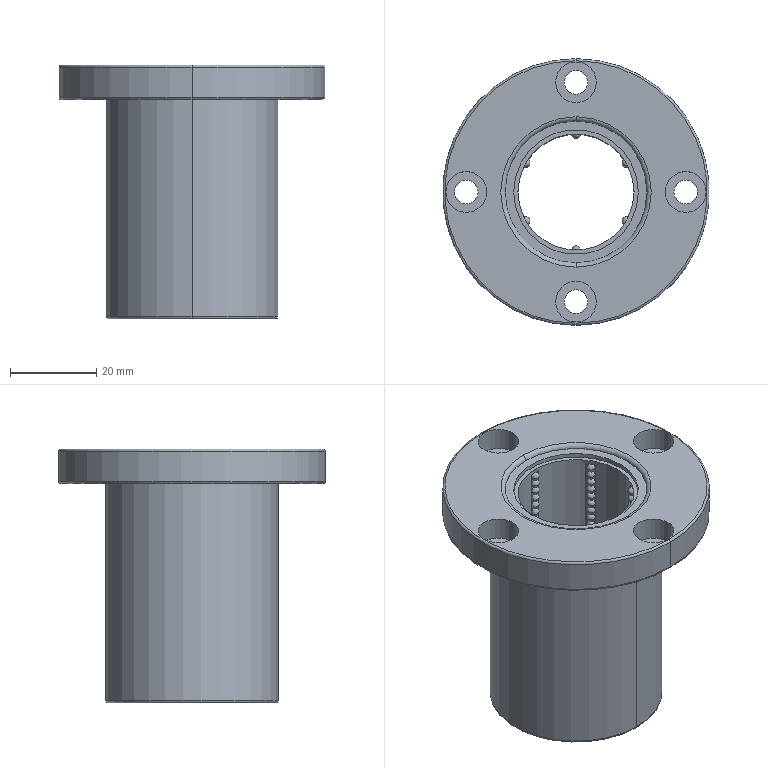Part | SolidWorks | features ICE 12, Fillet 2, Revolution 2, CirPattern 1, LPattern 1 | 1 solid | 383 faces | box 62 x 62 x 59 mm | volume 52518 mm3 | sphere 312 | plane 39 | cylinder 24 | torus 8 | commonest cylinder face diameters 5.5 x8 9.5 x8 26.99 x2 28.99 x2 40 x2 62 x2